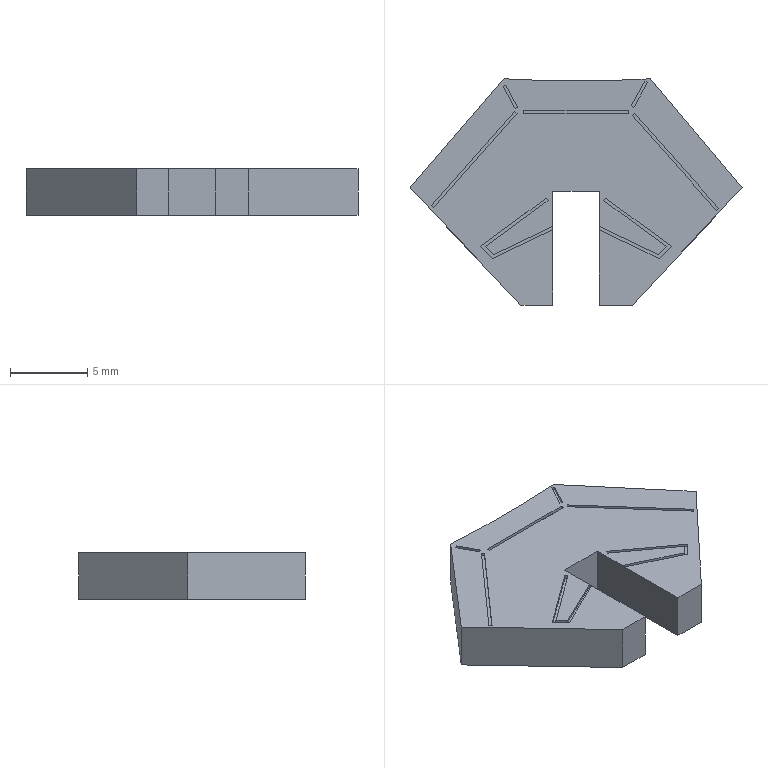Part | SolidWorks | features BaseBody 1 | 1 solid | 57 faces | box 21.443 x 14.616 x 3 mm | volume 580.976 mm3 | plane 51 | spline 6